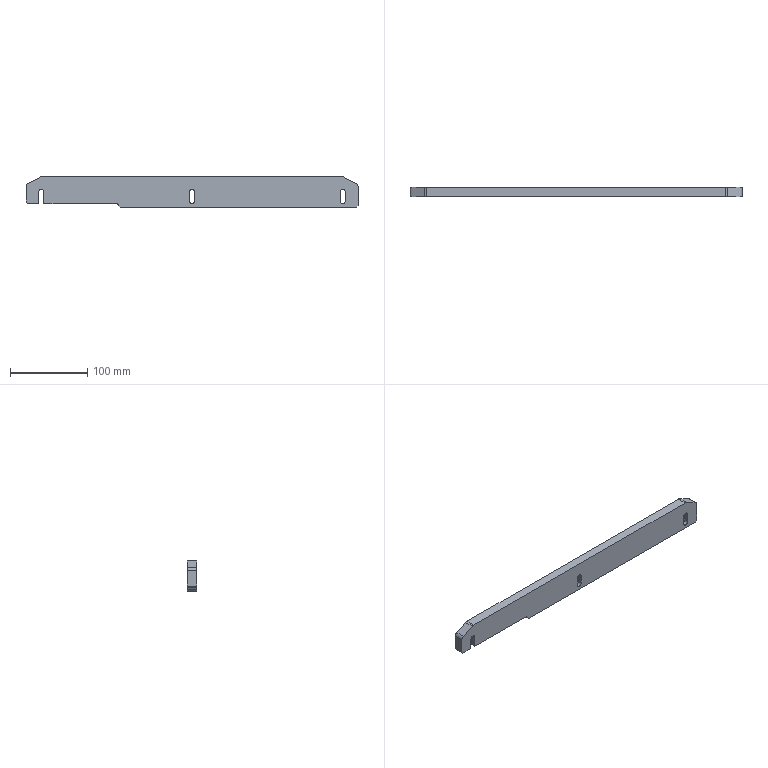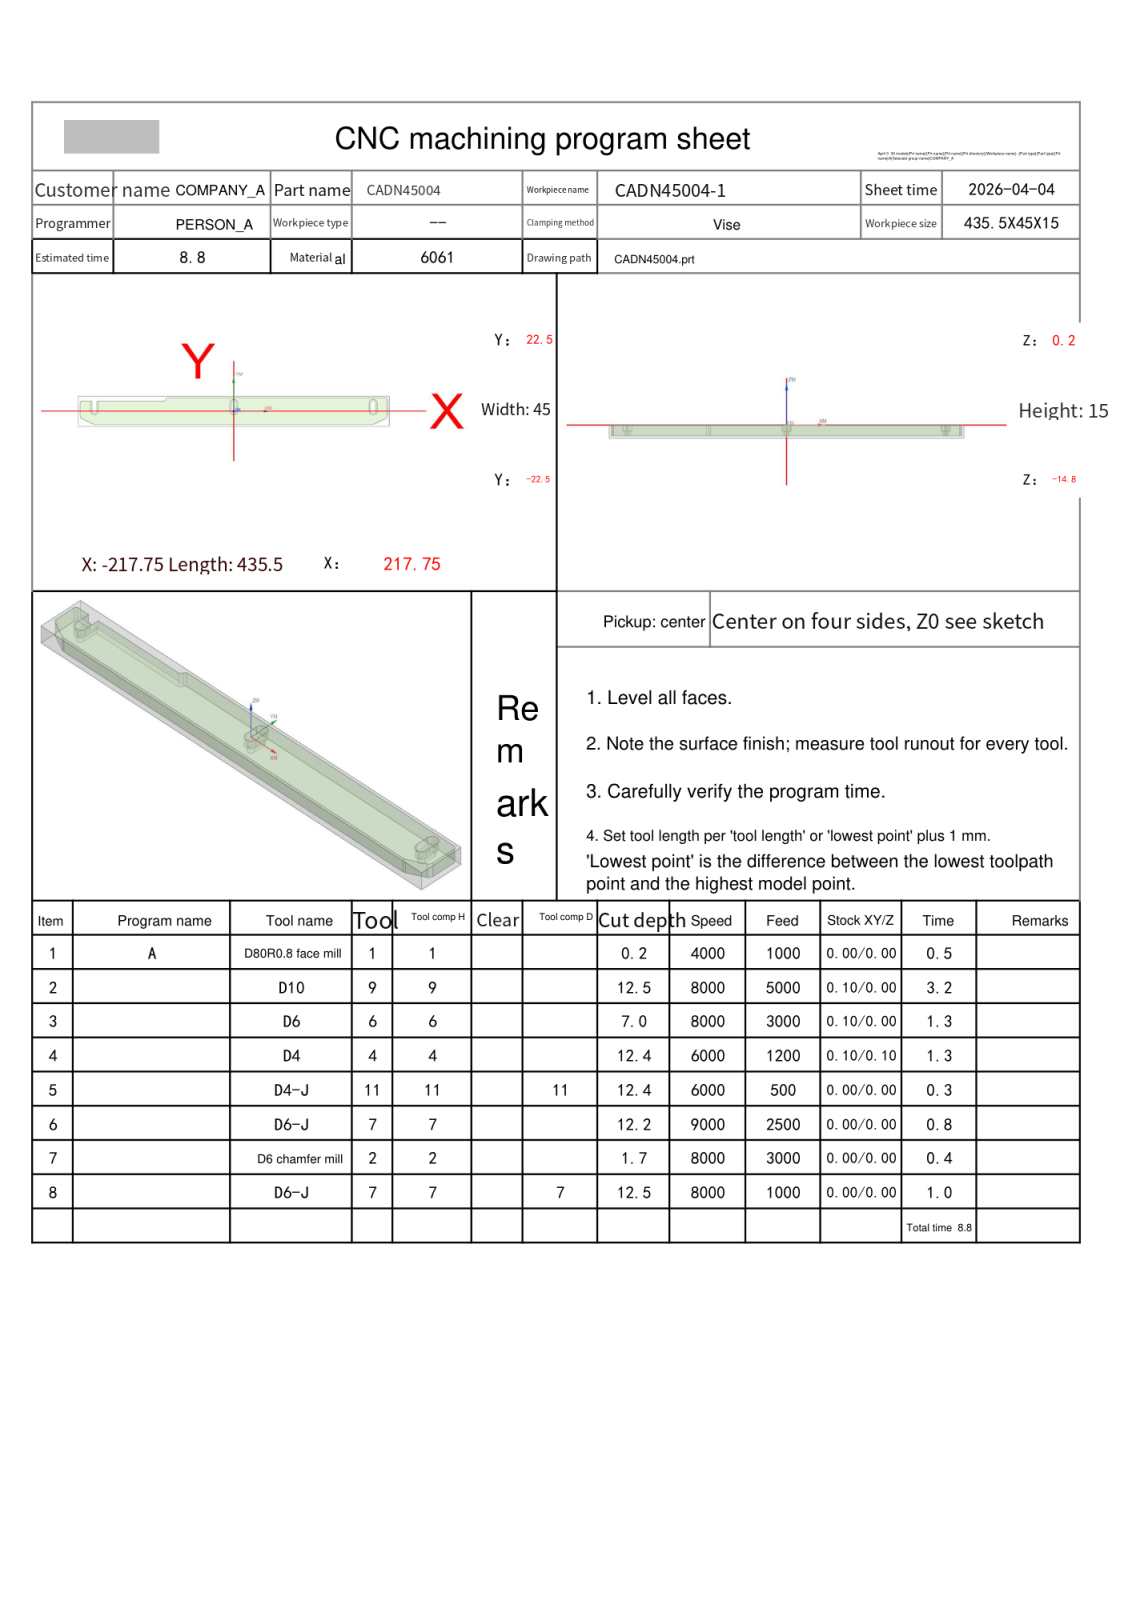NC program | NX | posted by the shop | part box 430.5 x 12 x 40 mm
Lines 1347 to 3269 of 3420, first 1495 of 1923 lines:
N6 T07 M06
(D6-J  D=6. R=0. H=07 ce=0.00 di=0.01)
G00 G90 G54 X-100.649 Y18.9 M03 S9000
G43 H07 Z20.
M08
Z.601
G01 X-100.648 Y18.89 Z.472 F2000.
X-100.643 Y18.861 Z.356
X-100.635 Y18.817 Z.251
X-100.623 Y18.759 Z.157
X-100.607 Y18.691 Z.073
X-100.586 Y18.615 Z0.0
X-100.56 Y18.534 Z-.064
X-100.529 Y18.45 Z-.119
X-100.492 Y18.366 Z-.165
X-100.45 Y18.285 Z-.204
X-100.401 Y18.209 Z-.235
X-100.345 Y18.141 Z-.259
X-100.283 Y18.083 Z-.277
X-100.213 Y18.039 Z-.29
X-100.135 Y18.01 Z-.297
X-100.049 Y18. Z-.299
X-98.25 F2500.
G02 X-97.875 Y19.452 I3. J0.0
G01 X-97.854 Y19.521 Z-.3
X-97.866 Y19.583 Z-.302
X-97.908 Y19.64 Z-.306
X-97.976 Y19.69 Z-.312
X-98.066 Y19.733 Z-.319
X-98.173 Y19.768 Z-.327
X-98.295 Y19.795 Z-.336
X-98.426 Y19.814 Z-.346
X-98.563 Y19.825 Z-.357
X-98.703 Y19.826 Z-.368
X-98.84 Y19.818 Z-.38
X-99.078 Y19.777 Z-.402
X-99.295 Y19.703 Z-.425
X-99.493 Y19.596 Z-.448
X-99.67 Y19.456 Z-.471
X-99.827 Y19.284 Z-.494
X-99.964 Y19.079 Z-.517
X-100.03 Y18.954 Z-.528
X-100.088 Y18.823 Z-.54
X-100.138 Y18.69 Z-.55
X-100.177 Y18.559 Z-.56
X-100.205 Y18.433 Z-.569
X-100.22 Y18.316 Z-.577
Y18.212 Z-.584
X-100.204 Y18.125 Z-.59
X-100.172 Y18.058 Z-.594
X-100.12 Y18.015 Z-.597
X-100.049 Y18. Z-.598
X-98.25
G02 X-97.875 Y19.452 I3. J0.0
G01 X-97.854 Y19.521
X-97.866 Y19.583 Z-.601
X-97.908 Y19.64 Z-.605
X-97.976 Y19.69 Z-.611
X-98.066 Y19.733 Z-.618
X-98.173 Y19.768 Z-.626
X-98.295 Y19.795 Z-.635
X-98.426 Y19.814 Z-.645
X-98.563 Y19.825 Z-.655
X-98.703 Y19.826 Z-.667
X-98.84 Y19.818 Z-.678
X-99.078 Y19.777 Z-.701
X-99.295 Y19.703 Z-.724
X-99.493 Y19.596 Z-.747
X-99.67 Y19.456 Z-.77
X-99.827 Y19.284 Z-.793
X-99.964 Y19.079 Z-.815
X-100.03 Y18.954 Z-.827
X-100.088 Y18.823 Z-.838
X-100.138 Y18.69 Z-.849
X-100.177 Y18.559 Z-.859
X-100.205 Y18.433 Z-.868
X-100.22 Y18.316 Z-.876
Y18.212 Z-.883
X-100.204 Y18.125 Z-.889
X-100.172 Y18.058 Z-.893
X-100.12 Y18.015 Z-.895
X-100.049 Y18. Z-.896
X-98.25
G02 X-97.875 Y19.452 I3. J0.0
G01 X-97.854 Y19.521 Z-.897
X-97.866 Y19.583 Z-.9
X-97.908 Y19.64 Z-.904
X-97.976 Y19.69 Z-.91
X-98.066 Y19.733 Z-.916
X-98.173 Y19.768 Z-.925
X-98.295 Y19.795 Z-.934
X-98.426 Y19.814 Z-.944
X-98.563 Y19.825 Z-.954
X-98.703 Y19.826 Z-.965
X-98.84 Y19.818 Z-.977
X-99.078 Y19.777 Z-.999
X-99.295 Y19.703 Z-1.022
X-99.493 Y19.596 Z-1.046
X-99.67 Y19.456 Z-1.069
X-99.827 Y19.284 Z-1.092
X-99.964 Y19.079 Z-1.114
X-100.03 Y18.954 Z-1.126
X-100.088 Y18.823 Z-1.137
X-100.138 Y18.69 Z-1.148
X-100.177 Y18.559 Z-1.158
X-100.205 Y18.433 Z-1.167
X-100.22 Y18.316 Z-1.175
Y18.212 Z-1.182
X-100.204 Y18.125 Z-1.187
X-100.172 Y18.058 Z-1.191
X-100.12 Y18.015 Z-1.194
X-100.049 Y18. Z-1.195
X-98.25
G02 X-97.875 Y19.452 I3. J0.0
G01 X-97.854 Y19.521 Z-1.196
X-97.866 Y19.583 Z-1.199
X-97.908 Y19.64 Z-1.203
X-97.976 Y19.69 Z-1.208
X-98.066 Y19.733 Z-1.215
X-98.173 Y19.768 Z-1.223
X-98.295 Y19.795 Z-1.232
X-98.426 Y19.814 Z-1.242
X-98.563 Y19.825 Z-1.253
X-98.703 Y19.826 Z-1.264
X-98.84 Y19.818 Z-1.276
X-99.078 Y19.777 Z-1.298
X-99.295 Y19.703 Z-1.321
X-99.493 Y19.596 Z-1.344
X-99.67 Y19.456 Z-1.368
X-99.827 Y19.284 Z-1.391
X-99.964 Y19.079 Z-1.413
X-100.03 Y18.954 Z-1.425
X-100.088 Y18.823 Z-1.436
X-100.138 Y18.69 Z-1.446
X-100.177 Y18.559 Z-1.456
X-100.205 Y18.433 Z-1.465
X-100.22 Y18.316 Z-1.474
Y18.212 Z-1.48
X-100.204 Y18.125 Z-1.486
X-100.172 Y18.058 Z-1.49
X-100.12 Y18.015 Z-1.493
X-100.049 Y18. Z-1.494
X-98.25
G02 X-97.875 Y19.452 I3. J0.0
G01 X-97.854 Y19.521 Z-1.495
X-97.866 Y19.583 Z-1.497
X-97.908 Y19.64 Z-1.501
X-97.976 Y19.69 Z-1.507
X-98.066 Y19.733 Z-1.514
X-98.173 Y19.768 Z-1.522
X-98.295 Y19.795 Z-1.531
X-98.426 Y19.814 Z-1.541
X-98.563 Y19.825 Z-1.552
X-98.703 Y19.826 Z-1.563
X-98.84 Y19.818 Z-1.575
X-99.078 Y19.777 Z-1.597
X-99.295 Y19.703 Z-1.62
X-99.493 Y19.596 Z-1.643
X-99.67 Y19.456 Z-1.666
X-99.827 Y19.284 Z-1.689
X-99.964 Y19.079 Z-1.712
X-100.03 Y18.954 Z-1.723
X-100.088 Y18.823 Z-1.735
X-100.138 Y18.69 Z-1.745
X-100.177 Y18.559 Z-1.755
X-100.205 Y18.433 Z-1.764
X-100.22 Y18.316 Z-1.772
Y18.212 Z-1.779
X-100.204 Y18.125 Z-1.785
X-100.172 Y18.058 Z-1.789
X-100.12 Y18.015 Z-1.792
X-100.049 Y18. Z-1.793
X-98.25
G02 X-97.875 Y19.452 I3. J0.0
G01 X-97.854 Y19.521
X-97.866 Y19.583 Z-1.796
X-97.908 Y19.64 Z-1.8
X-97.976 Y19.69 Z-1.806
X-98.066 Y19.733 Z-1.813
X-98.173 Y19.768 Z-1.821
X-98.295 Y19.795 Z-1.83
X-98.426 Y19.814 Z-1.84
X-98.563 Y19.825 Z-1.85
X-98.703 Y19.826 Z-1.862
X-98.84 Y19.818 Z-1.873
X-99.078 Y19.777 Z-1.896
X-99.295 Y19.703 Z-1.919
X-99.493 Y19.596 Z-1.942
X-99.67 Y19.456 Z-1.965
X-99.827 Y19.284 Z-1.988
X-99.964 Y19.079 Z-2.01
X-100.03 Y18.954 Z-2.022
X-100.088 Y18.823 Z-2.033
X-100.138 Y18.69 Z-2.044
X-100.177 Y18.559 Z-2.054
X-100.205 Y18.433 Z-2.063
X-100.22 Y18.316 Z-2.071
Y18.212 Z-2.078
X-100.204 Y18.125 Z-2.084
X-100.172 Y18.058 Z-2.088
X-100.12 Y18.015 Z-2.09
X-100.049 Y18. Z-2.091
X-98.25
G02 X-97.875 Y19.452 I3. J0.0
G01 X-97.854 Y19.521 Z-2.092
X-97.866 Y19.583 Z-2.095
X-97.908 Y19.64 Z-2.099
X-97.976 Y19.69 Z-2.105
X-98.066 Y19.733 Z-2.111
X-98.173 Y19.768 Z-2.12
X-98.295 Y19.795 Z-2.129
X-98.426 Y19.814 Z-2.139
X-98.563 Y19.825 Z-2.149
X-98.703 Y19.826 Z-2.16
X-98.84 Y19.818 Z-2.172
X-99.078 Y19.777 Z-2.194
X-99.295 Y19.703 Z-2.217
X-99.493 Y19.596 Z-2.241
X-99.67 Y19.456 Z-2.264
X-99.827 Y19.284 Z-2.287
X-99.964 Y19.079 Z-2.309
X-100.03 Y18.954 Z-2.321
X-100.088 Y18.823 Z-2.332
X-100.138 Y18.69 Z-2.343
X-100.177 Y18.559 Z-2.353
X-100.205 Y18.433 Z-2.362
X-100.22 Y18.316 Z-2.37
Y18.212 Z-2.377
X-100.204 Y18.125 Z-2.382
X-100.172 Y18.058 Z-2.386
X-100.12 Y18.015 Z-2.389
X-100.049 Y18. Z-2.39
X-98.25
G02 X-97.875 Y19.452 I3. J0.0
G01 X-97.854 Y19.521 Z-2.391
X-97.866 Y19.583 Z-2.394
X-97.908 Y19.64 Z-2.398
X-97.976 Y19.69 Z-2.403
X-98.066 Y19.733 Z-2.41
X-98.173 Y19.768 Z-2.418
X-98.295 Y19.795 Z-2.427
X-98.426 Y19.814 Z-2.437
X-98.563 Y19.825 Z-2.448
X-98.703 Y19.826 Z-2.459
X-98.84 Y19.818 Z-2.471
X-99.078 Y19.777 Z-2.493
X-99.295 Y19.703 Z-2.516
X-99.493 Y19.596 Z-2.539
X-99.67 Y19.456 Z-2.563
X-99.827 Y19.284 Z-2.586
X-99.964 Y19.079 Z-2.608
X-100.03 Y18.954 Z-2.62
X-100.088 Y18.823 Z-2.631
X-100.138 Y18.69 Z-2.641
X-100.177 Y18.559 Z-2.651
X-100.205 Y18.433 Z-2.66
X-100.22 Y18.316 Z-2.669
Y18.212 Z-2.675
X-100.204 Y18.125 Z-2.681
X-100.172 Y18.058 Z-2.685
X-100.12 Y18.015 Z-2.688
X-100.049 Y18. Z-2.689
X-98.25
G02 X-97.875 Y19.452 I3. J0.0
G01 X-97.854 Y19.521 Z-2.69
X-97.866 Y19.583 Z-2.692
X-97.908 Y19.64 Z-2.696
X-97.976 Y19.69 Z-2.702
X-98.066 Y19.733 Z-2.709
X-98.173 Y19.768 Z-2.717
X-98.295 Y19.795 Z-2.726
X-98.426 Y19.814 Z-2.736
X-98.563 Y19.825 Z-2.747
X-98.703 Y19.826 Z-2.758
X-98.84 Y19.818 Z-2.77
X-99.078 Y19.777 Z-2.792
X-99.295 Y19.703 Z-2.815
X-99.493 Y19.596 Z-2.838
X-99.67 Y19.456 Z-2.861
X-99.827 Y19.284 Z-2.884
X-99.964 Y19.079 Z-2.907
X-100.03 Y18.954 Z-2.918
X-100.088 Y18.823 Z-2.93
X-100.138 Y18.69 Z-2.94
X-100.177 Y18.559 Z-2.95
X-100.205 Y18.433 Z-2.959
X-100.22 Y18.316 Z-2.967
Y18.212 Z-2.974
X-100.204 Y18.125 Z-2.98
X-100.172 Y18.058 Z-2.984
X-100.12 Y18.015 Z-2.987
X-100.049 Y18. Z-2.988
X-98.25
G02 X-97.875 Y19.452 I3. J0.0
G01 X-97.854 Y19.521
X-97.866 Y19.583 Z-2.991
X-97.908 Y19.64 Z-2.995
X-97.976 Y19.69 Z-3.001
X-98.066 Y19.733 Z-3.008
X-98.173 Y19.768 Z-3.016
X-98.295 Y19.795 Z-3.025
X-98.426 Y19.814 Z-3.035
X-98.563 Y19.825 Z-3.045
X-98.703 Y19.826 Z-3.057
X-98.84 Y19.818 Z-3.068
X-99.078 Y19.777 Z-3.091
X-99.295 Y19.703 Z-3.114
X-99.493 Y19.596 Z-3.137
X-99.67 Y19.456 Z-3.16
X-99.827 Y19.284 Z-3.183
X-99.964 Y19.079 Z-3.205
X-100.03 Y18.954 Z-3.217
X-100.088 Y18.823 Z-3.228
X-100.138 Y18.69 Z-3.239
X-100.177 Y18.559 Z-3.249
X-100.205 Y18.433 Z-3.258
X-100.22 Y18.316 Z-3.266
Y18.212 Z-3.273
X-100.204 Y18.125 Z-3.279
X-100.172 Y18.058 Z-3.283
X-100.12 Y18.015 Z-3.285
X-100.049 Y18. Z-3.286
X-98.25
G02 X-97.875 Y19.452 I3. J0.0
G01 X-97.854 Y19.521 Z-3.287
X-97.866 Y19.583 Z-3.29
X-97.908 Y19.64 Z-3.294
X-97.976 Y19.69 Z-3.3
X-98.066 Y19.733 Z-3.306
X-98.173 Y19.768 Z-3.315
X-98.295 Y19.795 Z-3.324
X-98.426 Y19.814 Z-3.334
X-98.563 Y19.825 Z-3.344
X-98.703 Y19.826 Z-3.355
X-98.84 Y19.818 Z-3.367
X-99.078 Y19.777 Z-3.389
X-99.295 Y19.703 Z-3.412
X-99.493 Y19.596 Z-3.436
X-99.67 Y19.456 Z-3.459
X-99.827 Y19.284 Z-3.482
X-99.964 Y19.079 Z-3.504
X-100.03 Y18.954 Z-3.516
X-100.088 Y18.823 Z-3.527
X-100.138 Y18.69 Z-3.538
X-100.177 Y18.559 Z-3.548
X-100.205 Y18.433 Z-3.557
X-100.22 Y18.316 Z-3.565
Y18.212 Z-3.572
X-100.204 Y18.125 Z-3.577
X-100.172 Y18.058 Z-3.581
X-100.12 Y18.015 Z-3.584
X-100.049 Y18. Z-3.585
X-98.25
G02 X-97.875 Y19.452 I3. J0.0
G01 X-97.854 Y19.521 Z-3.586
X-97.866 Y19.583 Z-3.589
X-97.908 Y19.64 Z-3.593
X-97.976 Y19.69 Z-3.598
X-98.066 Y19.733 Z-3.605
X-98.173 Y19.768 Z-3.613
X-98.295 Y19.795 Z-3.622
X-98.426 Y19.814 Z-3.632
X-98.563 Y19.825 Z-3.643
X-98.703 Y19.826 Z-3.654
X-98.84 Y19.818 Z-3.666
X-99.078 Y19.777 Z-3.688
X-99.295 Y19.703 Z-3.711
X-99.493 Y19.596 Z-3.734
X-99.67 Y19.456 Z-3.758
X-99.827 Y19.284 Z-3.781
X-99.964 Y19.079 Z-3.803
X-100.03 Y18.954 Z-3.815
X-100.088 Y18.823 Z-3.826
X-100.138 Y18.69 Z-3.836
X-100.177 Y18.559 Z-3.846
X-100.205 Y18.433 Z-3.855
X-100.22 Y18.316 Z-3.864
Y18.212 Z-3.87
X-100.204 Y18.125 Z-3.876
X-100.172 Y18.058 Z-3.88
X-100.12 Y18.015 Z-3.883
X-100.049 Y18. Z-3.884
X-98.25
G02 X-97.875 Y19.452 I3. J0.0
G01 X-97.854 Y19.521 Z-3.885
X-97.866 Y19.583 Z-3.887
X-97.908 Y19.64 Z-3.891
X-97.976 Y19.69 Z-3.897
X-98.066 Y19.733 Z-3.904
X-98.173 Y19.768 Z-3.912
X-98.295 Y19.795 Z-3.921
X-98.426 Y19.814 Z-3.931
X-98.563 Y19.825 Z-3.942
X-98.703 Y19.826 Z-3.953
X-98.84 Y19.818 Z-3.965
X-99.078 Y19.777 Z-3.987
X-99.295 Y19.703 Z-4.01
X-99.493 Y19.596 Z-4.033
X-99.67 Y19.456 Z-4.056
X-99.827 Y19.284 Z-4.079
X-99.964 Y19.079 Z-4.102
X-100.03 Y18.954 Z-4.113
X-100.088 Y18.823 Z-4.125
X-100.138 Y18.69 Z-4.135
X-100.177 Y18.559 Z-4.145
X-100.205 Y18.433 Z-4.154
X-100.22 Y18.316 Z-4.162
Y18.212 Z-4.169
X-100.204 Y18.125 Z-4.175
X-100.172 Y18.058 Z-4.179
X-100.12 Y18.015 Z-4.182
X-100.049 Y18. Z-4.183
X-98.25
G02 X-97.875 Y19.452 I3. J0.0
G01 X-97.854 Y19.521
X-97.866 Y19.583 Z-4.186
X-97.908 Y19.64 Z-4.19
X-97.976 Y19.69 Z-4.196
X-98.066 Y19.733 Z-4.203
X-98.173 Y19.768 Z-4.211
X-98.295 Y19.795 Z-4.22
X-98.426 Y19.814 Z-4.23
X-98.563 Y19.825 Z-4.24
X-98.703 Y19.826 Z-4.252
X-98.84 Y19.818 Z-4.263
X-99.078 Y19.777 Z-4.286
X-99.295 Y19.703 Z-4.309
X-99.493 Y19.596 Z-4.332
X-99.67 Y19.456 Z-4.355
X-99.827 Y19.284 Z-4.378
X-99.964 Y19.079 Z-4.4
X-100.03 Y18.954 Z-4.412
X-100.088 Y18.823 Z-4.423
X-100.138 Y18.69 Z-4.434
X-100.177 Y18.559 Z-4.444
X-100.205 Y18.433 Z-4.453
X-100.22 Y18.316 Z-4.461
Y18.212 Z-4.468
X-100.204 Y18.125 Z-4.474
X-100.172 Y18.058 Z-4.478
X-100.12 Y18.015 Z-4.48
X-100.049 Y18. Z-4.481
X-98.25
G02 X-97.875 Y19.452 I3. J0.0
G01 X-97.854 Y19.521 Z-4.482
X-97.866 Y19.583 Z-4.485
X-97.908 Y19.64 Z-4.489
X-97.976 Y19.69 Z-4.495
X-98.066 Y19.733 Z-4.501
X-98.173 Y19.768 Z-4.51
X-98.295 Y19.795 Z-4.519
X-98.426 Y19.814 Z-4.529
X-98.563 Y19.825 Z-4.539
X-98.703 Y19.826 Z-4.55
X-98.84 Y19.818 Z-4.562
X-99.078 Y19.777 Z-4.584
X-99.295 Y19.703 Z-4.607
X-99.493 Y19.596 Z-4.631
X-99.67 Y19.456 Z-4.654
X-99.827 Y19.284 Z-4.677
X-99.964 Y19.079 Z-4.699
X-100.03 Y18.954 Z-4.711
X-100.088 Y18.823 Z-4.722
X-100.138 Y18.69 Z-4.733
X-100.177 Y18.559 Z-4.743
X-100.205 Y18.433 Z-4.752
X-100.22 Y18.316 Z-4.76
Y18.212 Z-4.767
X-100.204 Y18.125 Z-4.772
X-100.172 Y18.058 Z-4.776
X-100.12 Y18.015 Z-4.779
X-100.049 Y18. Z-4.78
X-98.25
G02 X-97.875 Y19.452 I3. J0.0
G01 X-97.854 Y19.521 Z-4.781
X-97.866 Y19.583 Z-4.784
X-97.908 Y19.64 Z-4.788
X-97.976 Y19.69 Z-4.793
X-98.066 Y19.733 Z-4.8
X-98.173 Y19.768 Z-4.808
X-98.295 Y19.795 Z-4.817
X-98.426 Y19.814 Z-4.827
X-98.563 Y19.825 Z-4.838
X-98.703 Y19.826 Z-4.849
X-98.84 Y19.818 Z-4.861
X-99.078 Y19.777 Z-4.883
X-99.295 Y19.703 Z-4.906
X-99.493 Y19.596 Z-4.929
X-99.67 Y19.456 Z-4.953
X-99.827 Y19.284 Z-4.976
X-99.964 Y19.079 Z-4.998
X-100.03 Y18.954 Z-5.01
X-100.088 Y18.823 Z-5.021
X-100.138 Y18.69 Z-5.031
X-100.177 Y18.559 Z-5.041
X-100.205 Y18.433 Z-5.05
X-100.22 Y18.316 Z-5.059
Y18.212 Z-5.065
X-100.204 Y18.125 Z-5.071
X-100.172 Y18.058 Z-5.075
X-100.12 Y18.015 Z-5.078
X-100.049 Y18. Z-5.079
X-98.25
G02 X-97.875 Y19.452 I3. J0.0
G01 X-97.854 Y19.521 Z-5.08
X-97.866 Y19.583 Z-5.082
X-97.908 Y19.64 Z-5.086
X-97.976 Y19.69 Z-5.092
X-98.066 Y19.733 Z-5.099
X-98.173 Y19.768 Z-5.107
X-98.295 Y19.795 Z-5.116
X-98.426 Y19.814 Z-5.126
X-98.563 Y19.825 Z-5.137
X-98.703 Y19.826 Z-5.148
X-98.84 Y19.818 Z-5.16
X-99.078 Y19.777 Z-5.182
X-99.295 Y19.703 Z-5.205
X-99.493 Y19.596 Z-5.228
X-99.67 Y19.456 Z-5.251
X-99.827 Y19.284 Z-5.274
X-99.964 Y19.079 Z-5.297
X-100.03 Y18.954 Z-5.308
X-100.088 Y18.823 Z-5.32
X-100.138 Y18.69 Z-5.33
X-100.177 Y18.559 Z-5.34
X-100.205 Y18.433 Z-5.349
X-100.22 Y18.316 Z-5.357
Y18.212 Z-5.364
X-100.204 Y18.125 Z-5.37
X-100.172 Y18.058 Z-5.374
X-100.12 Y18.015 Z-5.377
X-100.049 Y18. Z-5.378
X-98.25
G02 X-97.875 Y19.452 I3. J0.0
G01 X-97.854 Y19.521
X-97.866 Y19.583 Z-5.381
X-97.908 Y19.64 Z-5.385
X-97.976 Y19.69 Z-5.391
X-98.066 Y19.733 Z-5.398
X-98.173 Y19.768 Z-5.406
X-98.295 Y19.795 Z-5.415
X-98.426 Y19.814 Z-5.425
X-98.563 Y19.825 Z-5.435
X-98.703 Y19.826 Z-5.447
X-98.84 Y19.818 Z-5.458
X-99.078 Y19.777 Z-5.481
X-99.295 Y19.703 Z-5.504
X-99.493 Y19.596 Z-5.527
X-99.67 Y19.456 Z-5.55
X-99.827 Y19.284 Z-5.573
X-99.964 Y19.079 Z-5.595
X-100.03 Y18.954 Z-5.607
X-100.088 Y18.823 Z-5.618
X-100.138 Y18.69 Z-5.629
X-100.177 Y18.559 Z-5.639
X-100.205 Y18.433 Z-5.648
X-100.22 Y18.316 Z-5.656
Y18.212 Z-5.663
X-100.204 Y18.125 Z-5.669
X-100.172 Y18.058 Z-5.673
X-100.12 Y18.015 Z-5.675
X-100.049 Y18. Z-5.676
X-98.25
G02 X-97.875 Y19.452 I3. J0.0
G01 X-97.854 Y19.521 Z-5.677
X-97.866 Y19.583 Z-5.68
X-97.908 Y19.64 Z-5.684
X-97.976 Y19.69 Z-5.69
X-98.066 Y19.733 Z-5.696
X-98.173 Y19.768 Z-5.705
X-98.295 Y19.795 Z-5.714
X-98.426 Y19.814 Z-5.724
X-98.563 Y19.825 Z-5.734
X-98.703 Y19.826 Z-5.745
X-98.84 Y19.818 Z-5.757
X-99.078 Y19.777 Z-5.779
X-99.295 Y19.703 Z-5.802
X-99.493 Y19.596 Z-5.826
X-99.67 Y19.456 Z-5.849
X-99.827 Y19.284 Z-5.872
X-99.964 Y19.079 Z-5.894
X-100.03 Y18.954 Z-5.906
X-100.088 Y18.823 Z-5.917
X-100.138 Y18.69 Z-5.928
X-100.177 Y18.559 Z-5.938
X-100.205 Y18.433 Z-5.947
X-100.22 Y18.316 Z-5.955
Y18.212 Z-5.962
X-100.204 Y18.125 Z-5.967
X-100.172 Y18.058 Z-5.971
X-100.12 Y18.015 Z-5.974
X-100.049 Y18. Z-5.975
X-98.25
G02 X-97.875 Y19.452 I3. J0.0
G01 X-97.854 Y19.521 Z-5.976
X-97.866 Y19.583 Z-5.979
X-97.908 Y19.64 Z-5.983
X-97.976 Y19.69 Z-5.988
X-98.066 Y19.733 Z-5.995
X-98.173 Y19.768 Z-6.003
X-98.295 Y19.795 Z-6.012
X-98.426 Y19.814 Z-6.022
X-98.563 Y19.825 Z-6.033
X-98.703 Y19.826 Z-6.044
X-98.84 Y19.818 Z-6.056
X-99.078 Y19.777 Z-6.078
X-99.295 Y19.703 Z-6.101
X-99.493 Y19.596 Z-6.124
X-99.67 Y19.456 Z-6.148
X-99.827 Y19.284 Z-6.171
X-99.964 Y19.079 Z-6.193
X-100.03 Y18.954 Z-6.205
X-100.088 Y18.823 Z-6.216
X-100.138 Y18.69 Z-6.226
X-100.177 Y18.559 Z-6.236
X-100.205 Y18.433 Z-6.245
X-100.22 Y18.316 Z-6.254
Y18.212 Z-6.26
X-100.204 Y18.125 Z-6.266
X-100.172 Y18.058 Z-6.27
X-100.12 Y18.015 Z-6.273
X-100.049 Y18. Z-6.274
X-98.25
G02 X-97.875 Y19.452 I3. J0.0
G01 X-97.854 Y19.521 Z-6.275
X-97.866 Y19.583 Z-6.277
X-97.908 Y19.64 Z-6.281
X-97.976 Y19.69 Z-6.287
X-98.066 Y19.733 Z-6.294
X-98.173 Y19.768 Z-6.302
X-98.295 Y19.795 Z-6.311
X-98.426 Y19.814 Z-6.321
X-98.563 Y19.825 Z-6.332
X-98.703 Y19.826 Z-6.343
X-98.84 Y19.818 Z-6.355
X-99.078 Y19.777 Z-6.377
X-99.295 Y19.703 Z-6.4
X-99.493 Y19.596 Z-6.423
X-99.67 Y19.456 Z-6.446
X-99.827 Y19.284 Z-6.469
X-99.964 Y19.079 Z-6.492
X-100.03 Y18.954 Z-6.503
X-100.088 Y18.823 Z-6.515
X-100.138 Y18.69 Z-6.525
X-100.177 Y18.559 Z-6.535
X-100.205 Y18.433 Z-6.544
X-100.22 Y18.316 Z-6.552
Y18.212 Z-6.559
X-100.204 Y18.125 Z-6.565
X-100.172 Y18.058 Z-6.569
X-100.12 Y18.015 Z-6.572
X-100.049 Y18. Z-6.573
X-98.25
G02 X-97.875 Y19.452 I3. J0.0
G01 X-97.854 Y19.521
X-97.866 Y19.583 Z-6.576
X-97.908 Y19.64 Z-6.58
X-97.976 Y19.69 Z-6.586
X-98.066 Y19.733 Z-6.593
X-98.173 Y19.768 Z-6.601
X-98.295 Y19.795 Z-6.61
X-98.426 Y19.814 Z-6.62
X-98.563 Y19.825 Z-6.63
X-98.703 Y19.826 Z-6.642
X-98.84 Y19.818 Z-6.653
X-99.078 Y19.777 Z-6.676
X-99.295 Y19.703 Z-6.699
X-99.493 Y19.596 Z-6.722
X-99.67 Y19.456 Z-6.745
X-99.827 Y19.284 Z-6.768
X-99.964 Y19.079 Z-6.79
X-100.03 Y18.954 Z-6.802
X-100.088 Y18.823 Z-6.813
X-100.138 Y18.69 Z-6.824
X-100.177 Y18.559 Z-6.834
X-100.205 Y18.433 Z-6.843
X-100.22 Y18.316 Z-6.851
Y18.212 Z-6.858
X-100.204 Y18.125 Z-6.864
X-100.172 Y18.058 Z-6.868
X-100.12 Y18.015 Z-6.87
X-100.049 Y18. Z-6.871
X-98.25
G02 X-97.875 Y19.452 I3. J0.0
G01 X-97.854 Y19.521 Z-6.872
X-97.866 Y19.583 Z-6.875
X-97.908 Y19.64 Z-6.879
X-97.976 Y19.69 Z-6.885
X-98.066 Y19.733 Z-6.891
X-98.173 Y19.768 Z-6.9
X-98.295 Y19.795 Z-6.909
X-98.426 Y19.814 Z-6.919
X-98.563 Y19.825 Z-6.929
X-98.703 Y19.826 Z-6.94
X-98.84 Y19.818 Z-6.952
X-99.078 Y19.777 Z-6.974
X-99.295 Y19.703 Z-6.997
X-99.493 Y19.596 Z-7.021
X-99.67 Y19.456 Z-7.044
X-99.827 Y19.284 Z-7.067
X-99.964 Y19.079 Z-7.089
X-100.03 Y18.954 Z-7.101
X-100.088 Y18.823 Z-7.112
X-100.138 Y18.69 Z-7.123
X-100.177 Y18.559 Z-7.133
X-100.205 Y18.433 Z-7.142
X-100.22 Y18.316 Z-7.15
Y18.212 Z-7.157
X-100.204 Y18.125 Z-7.162
X-100.172 Y18.058 Z-7.166
X-100.12 Y18.015 Z-7.169
X-100.049 Y18. Z-7.17
X-98.25
G02 X-97.875 Y19.452 I3. J0.0
G01 X-97.854 Y19.521 Z-7.171
X-97.866 Y19.583 Z-7.174
X-97.908 Y19.64 Z-7.178
X-97.976 Y19.69 Z-7.183
X-98.066 Y19.733 Z-7.19
X-98.173 Y19.768 Z-7.198
X-98.295 Y19.795 Z-7.207
X-98.426 Y19.814 Z-7.217
X-98.563 Y19.825 Z-7.228
X-98.703 Y19.826 Z-7.239
X-98.84 Y19.818 Z-7.251
X-99.078 Y19.777 Z-7.273
X-99.295 Y19.703 Z-7.296
X-99.493 Y19.596 Z-7.319
X-99.67 Y19.456 Z-7.343
X-99.827 Y19.284 Z-7.366
X-99.964 Y19.079 Z-7.388
X-100.03 Y18.954 Z-7.4
X-100.088 Y18.823 Z-7.411
X-100.138 Y18.69 Z-7.421
X-100.177 Y18.559 Z-7.431
X-100.205 Y18.433 Z-7.44
X-100.22 Y18.316 Z-7.449
Y18.212 Z-7.455
X-100.204 Y18.125 Z-7.461
X-100.172 Y18.058 Z-7.465
X-100.12 Y18.015 Z-7.468
X-100.049 Y18. Z-7.469
X-98.25
G02 X-97.875 Y19.452 I3. J0.0
G01 X-97.854 Y19.521 Z-7.47
X-97.866 Y19.583 Z-7.472
X-97.908 Y19.64 Z-7.476
X-97.976 Y19.69 Z-7.482
X-98.066 Y19.733 Z-7.489
X-98.173 Y19.768 Z-7.497
X-98.295 Y19.795 Z-7.506
X-98.426 Y19.814 Z-7.516
X-98.563 Y19.825 Z-7.527
X-98.703 Y19.826 Z-7.538
X-98.84 Y19.818 Z-7.55
X-99.078 Y19.777 Z-7.572
X-99.295 Y19.703 Z-7.595
X-99.493 Y19.596 Z-7.618
X-99.67 Y19.456 Z-7.641
X-99.827 Y19.284 Z-7.664
X-99.964 Y19.079 Z-7.687
X-100.03 Y18.954 Z-7.698
X-100.088 Y18.823 Z-7.71
X-100.138 Y18.69 Z-7.72
X-100.177 Y18.559 Z-7.73
X-100.205 Y18.433 Z-7.739
X-100.22 Y18.316 Z-7.747
Y18.212 Z-7.754
X-100.204 Y18.125 Z-7.76
X-100.172 Y18.058 Z-7.764
X-100.12 Y18.015 Z-7.767
X-100.049 Y18. Z-7.768
X-98.25
G02 X-97.875 Y19.452 I3. J0.0
G01 X-97.854 Y19.521
X-97.866 Y19.583 Z-7.771
X-97.908 Y19.64 Z-7.775
X-97.976 Y19.69 Z-7.781
X-98.066 Y19.733 Z-7.788
X-98.173 Y19.768 Z-7.796
X-98.295 Y19.795 Z-7.805
X-98.426 Y19.814 Z-7.815
X-98.563 Y19.825 Z-7.825
X-98.703 Y19.826 Z-7.837
X-98.84 Y19.818 Z-7.848
X-99.078 Y19.777 Z-7.871
X-99.295 Y19.703 Z-7.894
X-99.493 Y19.596 Z-7.917
X-99.67 Y19.456 Z-7.94
X-99.827 Y19.284 Z-7.963
X-99.964 Y19.079 Z-7.985
X-100.03 Y18.954 Z-7.997
X-100.088 Y18.823 Z-8.008
X-100.138 Y18.69 Z-8.019
X-100.177 Y18.559 Z-8.029
X-100.205 Y18.433 Z-8.038
X-100.22 Y18.316 Z-8.046
Y18.212 Z-8.053
X-100.204 Y18.125 Z-8.059
X-100.172 Y18.058 Z-8.063
X-100.12 Y18.015 Z-8.065
X-100.049 Y18. Z-8.066
X-98.25
G02 X-97.875 Y19.452 I3. J0.0
G01 X-97.854 Y19.521 Z-8.067
X-97.866 Y19.583 Z-8.07
X-97.908 Y19.64 Z-8.074
X-97.976 Y19.69 Z-8.08
X-98.066 Y19.733 Z-8.086
X-98.173 Y19.768 Z-8.095
X-98.295 Y19.795 Z-8.104
X-98.426 Y19.814 Z-8.114
X-98.563 Y19.825 Z-8.124
X-98.703 Y19.826 Z-8.135
X-98.84 Y19.818 Z-8.147
X-99.078 Y19.777 Z-8.169
X-99.295 Y19.703 Z-8.192
X-99.493 Y19.596 Z-8.216
X-99.67 Y19.456 Z-8.239
X-99.827 Y19.284 Z-8.262
X-99.964 Y19.079 Z-8.284
X-100.03 Y18.954 Z-8.296
X-100.088 Y18.823 Z-8.307
X-100.138 Y18.69 Z-8.318
X-100.177 Y18.559 Z-8.328
X-100.205 Y18.433 Z-8.337
X-100.22 Y18.316 Z-8.345
Y18.212 Z-8.352
X-100.204 Y18.125 Z-8.357
X-100.172 Y18.058 Z-8.361
X-100.12 Y18.015 Z-8.364
X-100.049 Y18. Z-8.365
X-98.25
G02 X-97.875 Y19.452 I3. J0.0
G01 X-97.854 Y19.521 Z-8.366
X-97.866 Y19.583 Z-8.369
X-97.908 Y19.64 Z-8.373
X-97.976 Y19.69 Z-8.378
X-98.066 Y19.733 Z-8.385
X-98.173 Y19.768 Z-8.393
X-98.295 Y19.795 Z-8.402
X-98.426 Y19.814 Z-8.412
X-98.563 Y19.825 Z-8.423
X-98.703 Y19.826 Z-8.434
X-98.84 Y19.818 Z-8.446
X-99.078 Y19.777 Z-8.468
X-99.295 Y19.703 Z-8.491
X-99.493 Y19.596 Z-8.514
X-99.67 Y19.456 Z-8.538
X-99.827 Y19.284 Z-8.561
X-99.964 Y19.079 Z-8.583
X-100.03 Y18.954 Z-8.595
X-100.088 Y18.823 Z-8.606
X-100.138 Y18.69 Z-8.616
X-100.177 Y18.559 Z-8.626
X-100.205 Y18.433 Z-8.635
X-100.22 Y18.316 Z-8.644
Y18.212 Z-8.65
X-100.204 Y18.125 Z-8.656
X-100.172 Y18.058 Z-8.66
X-100.12 Y18.015 Z-8.663
X-100.049 Y18. Z-8.664
X-98.25
G02 X-97.875 Y19.452 I3. J0.0
G01 X-97.854 Y19.521 Z-8.665
X-97.866 Y19.583 Z-8.667
X-97.908 Y19.64 Z-8.671
X-97.976 Y19.69 Z-8.677
X-98.066 Y19.733 Z-8.684
X-98.173 Y19.768 Z-8.692
X-98.295 Y19.795 Z-8.701
X-98.426 Y19.814 Z-8.711
X-98.563 Y19.825 Z-8.722
X-98.703 Y19.826 Z-8.733
X-98.84 Y19.818 Z-8.745
X-99.078 Y19.777 Z-8.767
X-99.295 Y19.703 Z-8.79
X-99.493 Y19.596 Z-8.813
X-99.67 Y19.456 Z-8.836
X-99.827 Y19.284 Z-8.859
X-99.964 Y19.079 Z-8.882
X-100.03 Y18.954 Z-8.893
X-100.088 Y18.823 Z-8.905
X-100.138 Y18.69 Z-8.915
X-100.177 Y18.559 Z-8.925
X-100.205 Y18.433 Z-8.934
X-100.22 Y18.316 Z-8.942
Y18.212 Z-8.949
X-100.204 Y18.125 Z-8.955
X-100.172 Y18.058 Z-8.959
X-100.12 Y18.015 Z-8.962
X-100.049 Y18. Z-8.963
X-98.25
G02 X-97.875 Y19.452 I3. J0.0
G01 X-97.854 Y19.521
X-97.866 Y19.583 Z-8.966
X-97.908 Y19.64 Z-8.97
X-97.976 Y19.69 Z-8.976
X-98.066 Y19.733 Z-8.983
X-98.173 Y19.768 Z-8.991
X-98.295 Y19.795 Z-9.
X-98.426 Y19.814 Z-9.01
X-98.563 Y19.825 Z-9.02
X-98.703 Y19.826 Z-9.032
X-98.84 Y19.818 Z-9.043
X-99.078 Y19.777 Z-9.066
X-99.295 Y19.703 Z-9.089
X-99.493 Y19.596 Z-9.112
X-99.67 Y19.456 Z-9.135
X-99.827 Y19.284 Z-9.158
X-99.964 Y19.079 Z-9.18
X-100.03 Y18.954 Z-9.192
X-100.088 Y18.823 Z-9.203
X-100.138 Y18.69 Z-9.214
X-100.177 Y18.559 Z-9.224
X-100.205 Y18.433 Z-9.233
X-100.22 Y18.316 Z-9.241
Y18.212 Z-9.248
X-100.204 Y18.125 Z-9.254
X-100.172 Y18.058 Z-9.258
X-100.12 Y18.015 Z-9.26
X-100.049 Y18. Z-9.261
X-98.25
G02 X-97.875 Y19.452 I3. J0.0
G01 X-97.854 Y19.521 Z-9.262
X-97.866 Y19.583 Z-9.265
X-97.908 Y19.64 Z-9.269
X-97.976 Y19.69 Z-9.275
X-98.066 Y19.733 Z-9.281
X-98.173 Y19.768 Z-9.29
X-98.295 Y19.795 Z-9.299
X-98.426 Y19.814 Z-9.309
X-98.563 Y19.825 Z-9.319
X-98.703 Y19.826 Z-9.33
X-98.84 Y19.818 Z-9.342
X-99.078 Y19.777 Z-9.364
X-99.295 Y19.703 Z-9.387
X-99.493 Y19.596 Z-9.411
X-99.67 Y19.456 Z-9.434
X-99.827 Y19.284 Z-9.457
X-99.964 Y19.079 Z-9.479
X-100.03 Y18.954 Z-9.491
X-100.088 Y18.823 Z-9.502
X-100.138 Y18.69 Z-9.513
X-100.177 Y18.559 Z-9.523
X-100.205 Y18.433 Z-9.532
X-100.22 Y18.316 Z-9.54
Y18.212 Z-9.547
X-100.204 Y18.125 Z-9.552
X-100.172 Y18.058 Z-9.556
X-100.12 Y18.015 Z-9.559
X-100.049 Y18. Z-9.56
X-98.25
G02 X-97.875 Y19.452 I3. J0.0
G01 X-97.854 Y19.521 Z-9.561
X-97.866 Y19.583 Z-9.564
X-97.908 Y19.64 Z-9.568
X-97.976 Y19.69 Z-9.573
X-98.066 Y19.733 Z-9.58
X-98.173 Y19.768 Z-9.588
X-98.295 Y19.795 Z-9.597
X-98.426 Y19.814 Z-9.607
X-98.563 Y19.825 Z-9.618
X-98.703 Y19.826 Z-9.629
X-98.84 Y19.818 Z-9.641
X-99.078 Y19.777 Z-9.663
X-99.295 Y19.703 Z-9.686
X-99.493 Y19.596 Z-9.709
X-99.67 Y19.456 Z-9.733
X-99.827 Y19.284 Z-9.756
X-99.964 Y19.079 Z-9.778
X-100.03 Y18.954 Z-9.79
X-100.088 Y18.823 Z-9.801
X-100.138 Y18.69 Z-9.811
X-100.177 Y18.559 Z-9.821
X-100.205 Y18.433 Z-9.83
X-100.22 Y18.316 Z-9.839
Y18.212 Z-9.845
X-100.204 Y18.125 Z-9.851
X-100.172 Y18.058 Z-9.855
X-100.12 Y18.015 Z-9.858
X-100.049 Y18. Z-9.859
X-98.25
G02 X-97.875 Y19.452 I3. J0.0
G01 X-97.854 Y19.521 Z-9.86
X-97.866 Y19.583 Z-9.862
X-97.908 Y19.64 Z-9.866
X-97.976 Y19.69 Z-9.872
X-98.066 Y19.733 Z-9.879
X-98.173 Y19.768 Z-9.887
X-98.295 Y19.795 Z-9.896
X-98.426 Y19.814 Z-9.906
X-98.563 Y19.825 Z-9.917
X-98.703 Y19.826 Z-9.928
X-98.84 Y19.818 Z-9.94
X-99.078 Y19.777 Z-9.962
X-99.295 Y19.703 Z-9.985
X-99.493 Y19.596 Z-10.008
X-99.67 Y19.456 Z-10.031
X-99.827 Y19.284 Z-10.054
X-99.964 Y19.079 Z-10.077
X-100.03 Y18.954 Z-10.088
X-100.088 Y18.823 Z-10.1
X-100.138 Y18.69 Z-10.11
X-100.177 Y18.559 Z-10.12
X-100.205 Y18.433 Z-10.129
X-100.22 Y18.316 Z-10.137
Y18.212 Z-10.144
X-100.204 Y18.125 Z-10.15
X-100.172 Y18.058 Z-10.154
X-100.12 Y18.015 Z-10.157
X-100.049 Y18. Z-10.158
X-98.25
G02 X-97.875 Y19.452 I3. J0.0
G01 X-97.854 Y19.521
X-97.866 Y19.583 Z-10.161
X-97.908 Y19.64 Z-10.165
X-97.976 Y19.69 Z-10.171
X-98.066 Y19.733 Z-10.178
X-98.173 Y19.768 Z-10.186
X-98.295 Y19.795 Z-10.195
X-98.426 Y19.814 Z-10.205
X-98.563 Y19.825 Z-10.215
X-98.703 Y19.826 Z-10.227
X-98.84 Y19.818 Z-10.238
X-99.078 Y19.777 Z-10.261
X-99.295 Y19.703 Z-10.284
X-99.493 Y19.596 Z-10.307
X-99.67 Y19.456 Z-10.33
X-99.827 Y19.284 Z-10.353
X-99.964 Y19.079 Z-10.375
X-100.03 Y18.954 Z-10.387
X-100.088 Y18.823 Z-10.398
X-100.138 Y18.69 Z-10.409
X-100.177 Y18.559 Z-10.419
X-100.205 Y18.433 Z-10.428
X-100.22 Y18.316 Z-10.436
Y18.212 Z-10.443
X-100.204 Y18.125 Z-10.449
X-100.172 Y18.058 Z-10.453
X-100.12 Y18.015 Z-10.455
X-100.049 Y18. Z-10.456
X-98.25
G02 X-97.875 Y19.452 I3. J0.0
G01 X-97.854 Y19.521 Z-10.457
X-97.866 Y19.583 Z-10.46
X-97.908 Y19.64 Z-10.464
X-97.976 Y19.69 Z-10.47
X-98.066 Y19.733 Z-10.476
X-98.173 Y19.768 Z-10.485
X-98.295 Y19.795 Z-10.494
X-98.426 Y19.814 Z-10.504
X-98.563 Y19.825 Z-10.514
X-98.703 Y19.826 Z-10.525
X-98.84 Y19.818 Z-10.537
X-99.078 Y19.777 Z-10.559
X-99.295 Y19.703 Z-10.582
X-99.493 Y19.596 Z-10.606
X-99.67 Y19.456 Z-10.629
X-99.827 Y19.284 Z-10.652
X-99.964 Y19.079 Z-10.674
X-100.03 Y18.954 Z-10.686
X-100.088 Y18.823 Z-10.697
X-100.138 Y18.69 Z-10.708
X-100.177 Y18.559 Z-10.718
X-100.205 Y18.433 Z-10.727
X-100.22 Y18.316 Z-10.735
Y18.212 Z-10.742
X-100.204 Y18.125 Z-10.747
X-100.172 Y18.058 Z-10.751
X-100.12 Y18.015 Z-10.754
X-100.049 Y18. Z-10.755
X-98.25
G02 X-97.875 Y19.452 I3. J0.0
G01 X-97.854 Y19.521 Z-10.756
X-97.866 Y19.583 Z-10.759
X-97.908 Y19.64 Z-10.763
X-97.976 Y19.69 Z-10.768
X-98.066 Y19.733 Z-10.775
X-98.173 Y19.768 Z-10.783
X-98.295 Y19.795 Z-10.792
X-98.426 Y19.814 Z-10.802
X-98.563 Y19.825 Z-10.813
X-98.703 Y19.826 Z-10.824
X-98.84 Y19.818 Z-10.836
X-99.078 Y19.777 Z-10.858
X-99.295 Y19.703 Z-10.881
X-99.493 Y19.596 Z-10.904
X-99.67 Y19.456 Z-10.928
X-99.827 Y19.284 Z-10.951
X-99.964 Y19.079 Z-10.973
X-100.03 Y18.954 Z-10.985
X-100.088 Y18.823 Z-10.996
X-100.138 Y18.69 Z-11.006
X-100.177 Y18.559 Z-11.016
X-100.205 Y18.433 Z-11.025
X-100.22 Y18.316 Z-11.034
Y18.212 Z-11.04
X-100.204 Y18.125 Z-11.046
X-100.172 Y18.058 Z-11.05
X-100.12 Y18.015 Z-11.053
X-100.049 Y18. Z-11.054
X-98.25
G02 X-97.875 Y19.452 I3. J0.0
G01 X-97.854 Y19.521 Z-11.055
X-97.866 Y19.583 Z-11.057
X-97.908 Y19.64 Z-11.061
X-97.976 Y19.69 Z-11.067
X-98.066 Y19.733 Z-11.074
X-98.173 Y19.768 Z-11.082
X-98.295 Y19.795 Z-11.091
X-98.426 Y19.814 Z-11.101
X-98.563 Y19.825 Z-11.112
X-98.703 Y19.826 Z-11.123
X-98.84 Y19.818 Z-11.135
X-99.078 Y19.777 Z-11.157
X-99.295 Y19.703 Z-11.18
X-99.493 Y19.596 Z-11.203
X-99.67 Y19.456 Z-11.226
X-99.827 Y19.284 Z-11.249
X-99.964 Y19.079 Z-11.272
X-100.03 Y18.954 Z-11.283
X-100.088 Y18.823 Z-11.295
X-100.138 Y18.69 Z-11.305
X-100.177 Y18.559 Z-11.315
X-100.205 Y18.433 Z-11.324
X-100.22 Y18.316 Z-11.332
Y18.212 Z-11.339
X-100.204 Y18.125 Z-11.345
X-100.172 Y18.058 Z-11.349
X-100.12 Y18.015 Z-11.352
X-100.049 Y18. Z-11.353
X-98.25
G02 X-97.875 Y19.452 I3. J0.0
G01 X-97.854 Y19.521
X-97.866 Y19.583 Z-11.356
X-97.908 Y19.64 Z-11.36
X-97.976 Y19.69 Z-11.366
X-98.066 Y19.733 Z-11.373
X-98.173 Y19.768 Z-11.381
X-98.295 Y19.795 Z-11.39
X-98.426 Y19.814 Z-11.4
X-98.563 Y19.825 Z-11.41
X-98.703 Y19.826 Z-11.422
X-98.84 Y19.818 Z-11.433
X-99.078 Y19.777 Z-11.456
X-99.295 Y19.703 Z-11.479
X-99.493 Y19.596 Z-11.502
X-99.67 Y19.456 Z-11.525
X-99.827 Y19.284 Z-11.548
X-99.964 Y19.079 Z-11.57
X-100.03 Y18.954 Z-11.582
X-100.088 Y18.823 Z-11.593
X-100.138 Y18.69 Z-11.604
X-100.177 Y18.559 Z-11.614
X-100.205 Y18.433 Z-11.623
X-100.22 Y18.316 Z-11.631
Y18.212 Z-11.638
X-100.204 Y18.125 Z-11.644
X-100.172 Y18.058 Z-11.648
X-100.12 Y18.015 Z-11.65
X-100.049 Y18. Z-11.651
X-98.25
G02 X-97.875 Y19.452 I3. J0.0
G01 X-97.854 Y19.521 Z-11.652
X-97.866 Y19.583 Z-11.655
X-97.908 Y19.64 Z-11.659
X-97.976 Y19.69 Z-11.665
X-98.066 Y19.733 Z-11.671
X-98.173 Y19.768 Z-11.68
X-98.295 Y19.795 Z-11.689
X-98.426 Y19.814 Z-11.699
X-98.563 Y19.825 Z-11.709
X-98.703 Y19.826 Z-11.72
X-98.84 Y19.818 Z-11.732
X-99.078 Y19.777 Z-11.754
X-99.295 Y19.703 Z-11.777
X-99.493 Y19.596 Z-11.801
X-99.67 Y19.456 Z-11.824
X-99.827 Y19.284 Z-11.847
X-99.964 Y19.079 Z-11.869
X-100.03 Y18.954 Z-11.881
X-100.088 Y18.823 Z-11.892
X-100.138 Y18.69 Z-11.903
X-100.177 Y18.559 Z-11.913
X-100.205 Y18.433 Z-11.922
X-100.22 Y18.316 Z-11.93
Y18.212 Z-11.937
X-100.204 Y18.125 Z-11.942
X-100.172 Y18.058 Z-11.946
X-100.12 Y18.015 Z-11.949
X-100.049 Y18. Z-11.95
X-98.25
G02 X-97.875 Y19.452 I3. J0.0
G01 X-97.843 Y19.532 Z-11.948
X-97.831 Y19.613 Z-11.941
X-97.837 Y19.694 Z-11.929
X-97.859 Y19.776 Z-11.911
X-97.893 Y19.856 Z-11.886
X-97.938 Y19.933 Z-11.855
X-97.991 Y20.008 Z-11.816
X-98.049 Y20.079 Z-11.77
X-98.11 Y20.144 Z-11.715
X-98.171 Y20.204 Z-11.651
X-98.229 Y20.257 Z-11.578
X-98.283 Y20.303 Z-11.494
X-98.329 Y20.34 Z-11.4
X-98.365 Y20.367 Z-11.295
X-98.388 Y20.384 Z-11.179
X-98.397 Y20.39 Z-11.05
G00 Z-3.573
X-196.744 Y18.515
Z-5.971
G01 X-196.749 Y18.505 Z-6.1 F2000.
X-196.762 Y18.479 Z-6.217
X-196.781 Y18.439 Z-6.322
X-196.806 Y18.385 Z-6.416
X-196.833 Y18.32 Z-6.499
X-196.861 Y18.245 Z-6.572
X-196.888 Y18.164 Z-6.636
X-196.912 Y18.077 Z-6.691
X-196.932 Y17.988 Z-6.738
X-196.946 Y17.896 Z-6.776
X-196.951 Y17.806 Z-6.808
X-196.946 Y17.717 Z-6.832
X-196.929 Y17.634 Z-6.85
X-196.899 Y17.557 Z-6.862
X-196.853 Y17.488 Z-6.869
X-196.789 Y17.429 Z-6.871
G02 X-195.55 Y15. I-1.761 J-2.429 F2500.
G01 Y0.0
G03 X-195.25 Y-.3 I.3 J0.0
X-194.95 Y0.0 I0.0 J.3
G01 Y15.
G02 X-193.711 Y17.429 I3. J0.0
G01 X-193.663 Y17.484 Z-6.872
X-193.649 Y17.55 Z-6.875
X-193.666 Y17.625 Z-6.879
X-193.71 Y17.707 Z-6.885
X-193.778 Y17.794 Z-6.891
X-193.866 Y17.883 Z-6.9
X-193.971 Y17.972 Z-6.909
X-194.09 Y18.059 Z-6.919
X-194.219 Y18.142 Z-6.929
X-194.354 Y18.218 Z-6.94
X-194.492 Y18.285 Z-6.952
X-194.745 Y18.38 Z-6.974
X-194.997 Y18.436 Z-6.997
X-195.249 Y18.456 Z-7.021
X-195.5 Y18.437 Z-7.044
X-195.753 Y18.38 Z-7.067
X-196.006 Y18.286 Z-7.089
X-196.144 Y18.219 Z-7.101
X-196.279 Y18.143 Z-7.112
X-196.408 Y18.06 Z-7.123
X-196.527 Y17.973 Z-7.133
X-196.633 Y17.883 Z-7.142
X-196.721 Y17.794 Z-7.15
X-196.79 Y17.707 Z-7.157
X-196.834 Y17.625 Z-7.162
X-196.851 Y17.55 Z-7.166
X-196.837 Y17.484 Z-7.169
X-196.789 Y17.429 Z-7.17
G02 X-195.55 Y15. I-1.761 J-2.429
G01 Y0.0
G03 X-195.25 Y-.3 I.3 J0.0
X-194.95 Y0.0 I0.0 J.3
G01 Y15.
G02 X-193.711 Y17.429 I3. J0.0
G01 X-193.663 Y17.484 Z-7.171
X-193.649 Y17.55 Z-7.174
X-193.666 Y17.625 Z-7.178
X-193.71 Y17.707 Z-7.183
X-193.778 Y17.794 Z-7.19
X-193.866 Y17.883 Z-7.198
X-193.971 Y17.972 Z-7.207
X-194.09 Y18.059 Z-7.217
X-194.219 Y18.142 Z-7.228
X-194.354 Y18.218 Z-7.239
X-194.492 Y18.285 Z-7.251
X-194.745 Y18.38 Z-7.273
X-194.997 Y18.436 Z-7.296
X-195.249 Y18.456 Z-7.319
X-195.5 Y18.437 Z-7.343
X-195.753 Y18.38 Z-7.366
X-196.006 Y18.286 Z-7.388
X-196.144 Y18.219 Z-7.4
X-196.279 Y18.143 Z-7.411
X-196.408 Y18.06 Z-7.421
X-196.527 Y17.973 Z-7.431
X-196.633 Y17.883 Z-7.44
X-196.721 Y17.794 Z-7.449
X-196.79 Y17.707 Z-7.455
X-196.834 Y17.625 Z-7.461
X-196.851 Y17.55 Z-7.465
X-196.837 Y17.484 Z-7.468
X-196.789 Y17.429 Z-7.469
G02 X-195.55 Y15. I-1.761 J-2.429
G01 Y0.0
G03 X-195.25 Y-.3 I.3 J0.0
X-194.95 Y0.0 I0.0 J.3
G01 Y15.
G02 X-193.711 Y17.429 I3. J0.0
G01 X-193.663 Y17.484 Z-7.47
X-193.649 Y17.55 Z-7.472
X-193.666 Y17.625 Z-7.476
X-193.71 Y17.707 Z-7.482
X-193.778 Y17.794 Z-7.489
X-193.866 Y17.883 Z-7.497
X-193.971 Y17.972 Z-7.506
X-194.09 Y18.059 Z-7.516
X-194.219 Y18.142 Z-7.527
X-194.354 Y18.218 Z-7.538
X-194.492 Y18.285 Z-7.55
X-194.745 Y18.38 Z-7.572
X-194.997 Y18.436 Z-7.595
X-195.249 Y18.456 Z-7.618
X-195.5 Y18.437 Z-7.641
X-195.753 Y18.38 Z-7.664
X-196.006 Y18.286 Z-7.687
X-196.144 Y18.219 Z-7.698
X-196.279 Y18.143 Z-7.71
X-196.408 Y18.06 Z-7.72
X-196.527 Y17.973 Z-7.73
X-196.633 Y17.883 Z-7.739
X-196.721 Y17.794 Z-7.747
X-196.79 Y17.707 Z-7.754
X-196.834 Y17.625 Z-7.76
X-196.851 Y17.55 Z-7.764
X-196.837 Y17.484 Z-7.767
X-196.789 Y17.429 Z-7.768
G02 X-195.55 Y15. I-1.761 J-2.429
G01 Y0.0
G03 X-195.25 Y-.3 I.3 J0.0
X-194.95 Y0.0 I0.0 J.3
G01 Y15.
G02 X-193.711 Y17.429 I3. J0.0
G01 X-193.663 Y17.484
X-193.649 Y17.55 Z-7.771
X-193.666 Y17.625 Z-7.775
X-193.71 Y17.707 Z-7.781
X-193.778 Y17.794 Z-7.788
X-193.866 Y17.883 Z-7.796
X-193.971 Y17.972 Z-7.805
X-194.09 Y18.059 Z-7.815
X-194.219 Y18.142 Z-7.825
X-194.354 Y18.218 Z-7.837
X-194.492 Y18.285 Z-7.848
X-194.745 Y18.38 Z-7.871
X-194.997 Y18.436 Z-7.894
X-195.249 Y18.456 Z-7.917
X-195.5 Y18.437 Z-7.94
X-195.753 Y18.38 Z-7.963
X-196.006 Y18.286 Z-7.985
X-196.144 Y18.219 Z-7.997
X-196.279 Y18.143 Z-8.008
X-196.408 Y18.06 Z-8.019
X-196.527 Y17.973 Z-8.029
X-196.633 Y17.883 Z-8.038
X-196.721 Y17.794 Z-8.046
X-196.79 Y17.707 Z-8.053
X-196.834 Y17.625 Z-8.059
X-196.851 Y17.55 Z-8.063
X-196.837 Y17.484 Z-8.065
X-196.789 Y17.429 Z-8.066
G02 X-195.55 Y15. I-1.761 J-2.429
G01 Y0.0
G03 X-195.25 Y-.3 I.3 J0.0
X-194.95 Y0.0 I0.0 J.3
G01 Y15.
G02 X-193.711 Y17.429 I3. J0.0
G01 X-193.663 Y17.484 Z-8.067
X-193.649 Y17.55 Z-8.07
X-193.666 Y17.625 Z-8.074
X-193.71 Y17.707 Z-8.08
X-193.778 Y17.794 Z-8.086
X-193.866 Y17.883 Z-8.095
X-193.971 Y17.972 Z-8.104
X-194.09 Y18.059 Z-8.114
X-194.219 Y18.142 Z-8.124
X-194.354 Y18.218 Z-8.135
X-194.492 Y18.285 Z-8.147
X-194.745 Y18.38 Z-8.169
X-194.997 Y18.436 Z-8.192
X-195.249 Y18.456 Z-8.216
X-195.5 Y18.437 Z-8.239
X-195.753 Y18.38 Z-8.262
X-196.006 Y18.286 Z-8.284
X-196.144 Y18.219 Z-8.296
X-196.279 Y18.143 Z-8.307
X-196.408 Y18.06 Z-8.318
X-196.527 Y17.973 Z-8.328
X-196.633 Y17.883 Z-8.337
X-196.721 Y17.794 Z-8.345
X-196.79 Y17.707 Z-8.352
X-196.834 Y17.625 Z-8.357
X-196.851 Y17.55 Z-8.361
X-196.837 Y17.484 Z-8.364
X-196.789 Y17.429 Z-8.365
G02 X-195.55 Y15. I-1.761 J-2.429
G01 Y0.0
G03 X-195.25 Y-.3 I.3 J0.0
X-194.95 Y0.0 I0.0 J.3
G01 Y15.
G02 X-193.711 Y17.429 I3. J0.0
G01 X-193.663 Y17.484 Z-8.366
X-193.649 Y17.55 Z-8.369
X-193.666 Y17.625 Z-8.373
X-193.71 Y17.707 Z-8.378
X-193.778 Y17.794 Z-8.385
X-193.866 Y17.883 Z-8.393
X-193.971 Y17.972 Z-8.402
X-194.09 Y18.059 Z-8.412
X-194.219 Y18.142 Z-8.423
X-194.354 Y18.218 Z-8.434
X-194.492 Y18.285 Z-8.446
X-194.745 Y18.38 Z-8.468
X-194.997 Y18.436 Z-8.491
X-195.249 Y18.456 Z-8.514
X-195.5 Y18.437 Z-8.538
X-195.753 Y18.38 Z-8.561
X-196.006 Y18.286 Z-8.583
X-196.144 Y18.219 Z-8.595
X-196.279 Y18.143 Z-8.606
X-196.408 Y18.06 Z-8.616
X-196.527 Y17.973 Z-8.626
X-196.633 Y17.883 Z-8.635
X-196.721 Y17.794 Z-8.644
X-196.79 Y17.707 Z-8.65
X-196.834 Y17.625 Z-8.656
X-196.851 Y17.55 Z-8.66
X-196.837 Y17.484 Z-8.663
X-196.789 Y17.429 Z-8.664
G02 X-195.55 Y15. I-1.761 J-2.429
G01 Y0.0
G03 X-195.25 Y-.3 I.3 J0.0
X-194.95 Y0.0 I0.0 J.3
G01 Y15.
G02 X-193.711 Y17.429 I3. J0.0
G01 X-193.663 Y17.484 Z-8.665
X-193.649 Y17.55 Z-8.667
X-193.666 Y17.625 Z-8.671
X-193.71 Y17.707 Z-8.677
X-193.778 Y17.794 Z-8.684
X-193.866 Y17.883 Z-8.692
X-193.971 Y17.972 Z-8.701
X-194.09 Y18.059 Z-8.711
X-194.219 Y18.142 Z-8.722
X-194.354 Y18.218 Z-8.733
X-194.492 Y18.285 Z-8.745
X-194.745 Y18.38 Z-8.767
X-194.997 Y18.436 Z-8.79
X-195.249 Y18.456 Z-8.813
X-195.5 Y18.437 Z-8.836
X-195.753 Y18.38 Z-8.859
X-196.006 Y18.286 Z-8.882
X-196.144 Y18.219 Z-8.893
X-196.279 Y18.143 Z-8.905
X-196.408 Y18.06 Z-8.915
X-196.527 Y17.973 Z-8.925
X-196.633 Y17.883 Z-8.934
X-196.721 Y17.794 Z-8.942
X-196.79 Y17.707 Z-8.949
X-196.834 Y17.625 Z-8.955
X-196.851 Y17.55 Z-8.959
X-196.837 Y17.484 Z-8.962
X-196.789 Y17.429 Z-8.963
G02 X-195.55 Y15. I-1.761 J-2.429
G01 Y0.0
G03 X-195.25 Y-.3 I.3 J0.0
X-194.95 Y0.0 I0.0 J.3
G01 Y15.
G02 X-193.711 Y17.429 I3. J0.0
G01 X-193.663 Y17.484
X-193.649 Y17.55 Z-8.966
X-193.666 Y17.625 Z-8.97
X-193.71 Y17.707 Z-8.976
X-193.778 Y17.794 Z-8.983
X-193.866 Y17.883 Z-8.991
X-193.971 Y17.972 Z-9.
X-194.09 Y18.059 Z-9.01
X-194.219 Y18.142 Z-9.02
X-194.354 Y18.218 Z-9.032
X-194.492 Y18.285 Z-9.043
X-194.745 Y18.38 Z-9.066
X-194.997 Y18.436 Z-9.089
X-195.249 Y18.456 Z-9.112
X-195.5 Y18.437 Z-9.135
X-195.753 Y18.38 Z-9.158
X-196.006 Y18.286 Z-9.18
X-196.144 Y18.219 Z-9.192
X-196.279 Y18.143 Z-9.203
X-196.408 Y18.06 Z-9.214
X-196.527 Y17.973 Z-9.224
X-196.633 Y17.883 Z-9.233